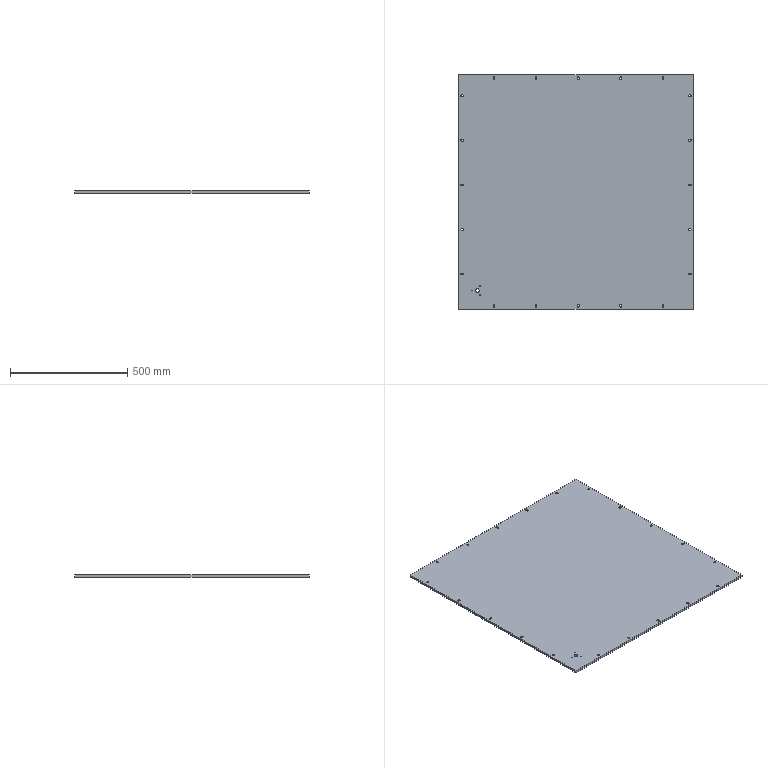Part | STEP file | SynoNew-0304-055 | 1 solid | 90 faces | box 1000 x 1000 x 10 mm | volume 9984549 mm3 | plane 46 | cylinder 44 | commonest cylinder face diameters 6.6 x40 3.2 x3 15 x1